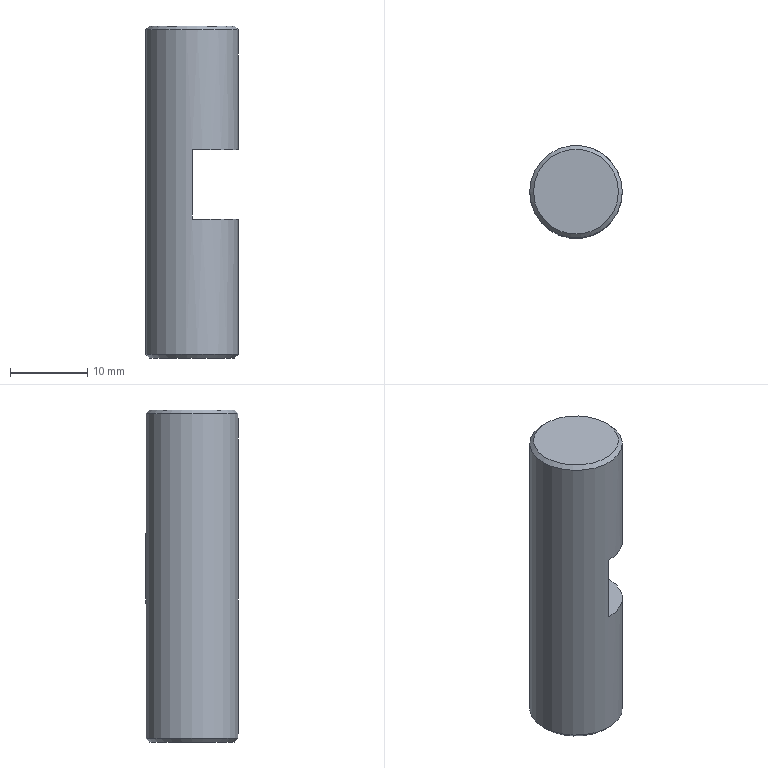Part | NX | features DATUM_CSYS 2, CHAMFER 1, CYLINDER 1, EXTRUDE 1, SKETCH 1 | 1 solid | 8 faces | box 12 x 12 x 43 mm | volume 4345 mm3 | plane 5 | cone 2 | cylinder 1 | commonest cylinder face diameters 12 x1
STEP:
#1=CARTESIAN_POINT('',(6.,0.,42.5));
#2=VERTEX_POINT('',#1);
#3=CARTESIAN_POINT('',(0.,0.,42.5));
#4=DIRECTION('',(0.,0.,1.));
#5=DIRECTION('',(1.,0.,0.));
#6=AXIS2_PLACEMENT_3D('',#3,#4,#5);
#7=CIRCLE('',#6,6.);
#8=EDGE_CURVE('',#2,#2,#7,.F.);
#9=ORIENTED_EDGE('',*,*,#8,.T.);
#10=EDGE_LOOP('',(#9));
#11=FACE_BOUND('',#10,.T.);
#12=CARTESIAN_POINT('',(-6.,0.,0.5));
#13=VERTEX_POINT('',#12);
#14=CARTESIAN_POINT('',(0.,0.,0.5));
#15=DIRECTION('',(0.,0.,-1.));
#16=DIRECTION('',(-1.,0.,0.));
#17=AXIS2_PLACEMENT_3D('',#14,#15,#16);
#18=CIRCLE('',#17,6.);
#19=EDGE_CURVE('',#13,#13,#18,.F.);
#20=ORIENTED_EDGE('',*,*,#19,.T.);
#21=EDGE_LOOP('',(#20));
#22=FACE_BOUND('',#21,.T.);
#23=CARTESIAN_POINT('',(0.,-6.,27.));
#24=VERTEX_POINT('',#23);
#25=CARTESIAN_POINT('',(0.,-6.,18.));
#26=VERTEX_POINT('',#25);
#27=CARTESIAN_POINT('',(0.,-6.,0.));
#28=DIRECTION('',(0.,0.,1.));
#29=VECTOR('',#28,1000.);
#30=LINE('',#27,#29);
#31=EDGE_CURVE('',#24,#26,#30,.F.);
#32=ORIENTED_EDGE('',*,*,#31,.F.);
#33=CARTESIAN_POINT('',(0.,6.,27.));
#34=VERTEX_POINT('',#33);
#35=CARTESIAN_POINT('',(0.,0.,27.));
#36=DIRECTION('',(0.,0.,-1.));
#37=DIRECTION('',(0.,1.,0.));
#38=AXIS2_PLACEMENT_3D('',#35,#36,#37);
#39=CIRCLE('',#38,6.);
#40=EDGE_CURVE('',#24,#34,#39,.F.);
#41=ORIENTED_EDGE('',*,*,#40,.T.);
#42=CARTESIAN_POINT('',(0.,6.,18.));
#43=VERTEX_POINT('',#42);
#44=CARTESIAN_POINT('',(0.,6.,0.));
#45=DIRECTION('',(0.,0.,1.));
#46=VECTOR('',#45,1000.);
#47=LINE('',#44,#46);
#48=EDGE_CURVE('',#43,#34,#47,.T.);
#49=ORIENTED_EDGE('',*,*,#48,.F.);
#50=CARTESIAN_POINT('',(0.,0.,18.));
#51=DIRECTION('',(0.,0.,1.));
#52=DIRECTION('',(1.,0.,0.));
#53=AXIS2_PLACEMENT_3D('',#50,#51,#52);
#54=CIRCLE('',#53,6.);
#55=EDGE_CURVE('',#43,#26,#54,.F.);
#56=ORIENTED_EDGE('',*,*,#55,.T.);
#57=EDGE_LOOP('',(#32,#41,#49,#56));
#58=FACE_BOUND('',#57,.T.);
#59=CARTESIAN_POINT('',(0.,0.,0.));
#60=DIRECTION('',(0.,0.,1.));
#61=DIRECTION('',(1.,0.,0.));
#62=AXIS2_PLACEMENT_3D('',#59,#60,#61);
#63=CYLINDRICAL_SURFACE('',#62,6.);
#64=ADVANCED_FACE('',(#11,#22,#58),#63,.T.);
#65=CARTESIAN_POINT('',(5.5,0.,43.));
#66=VERTEX_POINT('',#65);
#67=CARTESIAN_POINT('',(0.,0.,43.));
#68=DIRECTION('',(0.,0.,1.));
#69=DIRECTION('',(1.,0.,0.));
#70=AXIS2_PLACEMENT_3D('',#67,#68,#69);
#71=CIRCLE('',#70,5.5);
#72=EDGE_CURVE('',#66,#66,#71,.T.);
#73=ORIENTED_EDGE('',*,*,#72,.T.);
#74=EDGE_LOOP('',(#73));
#75=FACE_BOUND('',#74,.T.);
#76=CARTESIAN_POINT('',(0.,0.,43.));
#77=DIRECTION('',(0.,0.,1.));
#78=DIRECTION('',(1.,0.,0.));
#79=AXIS2_PLACEMENT_3D('',#76,#77,#78);
#80=PLANE('',#79);
#81=ADVANCED_FACE('',(#75),#80,.T.);
#82=CARTESIAN_POINT('',(-5.5,0.,0.));
#83=VERTEX_POINT('',#82);
#84=CARTESIAN_POINT('',(0.,0.,0.));
#85=DIRECTION('',(0.,0.,-1.));
#86=DIRECTION('',(-1.,0.,0.));
#87=AXIS2_PLACEMENT_3D('',#84,#85,#86);
#88=CIRCLE('',#87,5.5);
#89=EDGE_CURVE('',#83,#83,#88,.T.);
#90=ORIENTED_EDGE('',*,*,#89,.T.);
#91=EDGE_LOOP('',(#90));
#92=FACE_BOUND('',#91,.T.);
#93=CARTESIAN_POINT('',(0.,0.,0.));
#94=DIRECTION('',(0.,0.,-1.));
#95=DIRECTION('',(-1.,0.,0.));
#96=AXIS2_PLACEMENT_3D('',#93,#94,#95);
#97=PLANE('',#96);
#98=ADVANCED_FACE('',(#92),#97,.T.);
#99=ORIENTED_EDGE('',*,*,#72,.F.);
#100=EDGE_LOOP('',(#99));
#101=FACE_BOUND('',#100,.T.);
#102=ORIENTED_EDGE('',*,*,#8,.F.);
#103=EDGE_LOOP('',(#102));
#104=FACE_BOUND('',#103,.T.);
#105=CARTESIAN_POINT('',(0.,0.,42.5));
#106=DIRECTION('',(0.,0.,-1.));
#107=DIRECTION('',(-1.,0.,0.));
#108=AXIS2_PLACEMENT_3D('',#105,#106,#107);
#109=CONICAL_SURFACE('',#108,6.,0.7854);
#110=ADVANCED_FACE('',(#101,#104),#109,.T.);
#111=ORIENTED_EDGE('',*,*,#89,.F.);
#112=EDGE_LOOP('',(#111));
#113=FACE_BOUND('',#112,.T.);
#114=ORIENTED_EDGE('',*,*,#19,.F.);
#115=EDGE_LOOP('',(#114));
#116=FACE_BOUND('',#115,.T.);
#117=CARTESIAN_POINT('',(0.,0.,0.5));
#118=DIRECTION('',(0.,0.,1.));
#119=DIRECTION('',(1.,0.,0.));
#120=AXIS2_PLACEMENT_3D('',#117,#118,#119);
#121=CONICAL_SURFACE('',#120,6.,0.7854);
#122=ADVANCED_FACE('',(#113,#116),#121,.T.);
#123=CARTESIAN_POINT('',(0.,-17.217,27.));
#124=DIRECTION('',(0.,1.,0.));
#125=VECTOR('',#124,1000.);
#126=LINE('',#123,#125);
#127=EDGE_CURVE('',#34,#24,#126,.F.);
#128=ORIENTED_EDGE('',*,*,#127,.F.);
#129=ORIENTED_EDGE('',*,*,#40,.F.);
#130=EDGE_LOOP('',(#128,#129));
#131=FACE_BOUND('',#130,.T.);
#132=CARTESIAN_POINT('',(0.,-17.217,27.));
#133=DIRECTION('',(0.,0.,-1.));
#134=DIRECTION('',(0.,1.,0.));
#135=AXIS2_PLACEMENT_3D('',#132,#133,#134);
#136=PLANE('',#135);
#137=ADVANCED_FACE('',(#131),#136,.T.);
#138=ORIENTED_EDGE('',*,*,#55,.F.);
#139=CARTESIAN_POINT('',(0.,18.,18.));
#140=DIRECTION('',(0.,-1.,0.));
#141=VECTOR('',#140,1000.);
#142=LINE('',#139,#141);
#143=EDGE_CURVE('',#26,#43,#142,.F.);
#144=ORIENTED_EDGE('',*,*,#143,.F.);
#145=EDGE_LOOP('',(#138,#144));
#146=FACE_BOUND('',#145,.T.);
#147=CARTESIAN_POINT('',(0.,18.,18.));
#148=DIRECTION('',(0.,0.,1.));
#149=DIRECTION('',(1.,0.,0.));
#150=AXIS2_PLACEMENT_3D('',#147,#148,#149);
#151=PLANE('',#150);
#152=ADVANCED_FACE('',(#146),#151,.T.);
#153=ORIENTED_EDGE('',*,*,#31,.T.);
#154=ORIENTED_EDGE('',*,*,#143,.T.);
#155=ORIENTED_EDGE('',*,*,#48,.T.);
#156=ORIENTED_EDGE('',*,*,#127,.T.);
#157=EDGE_LOOP('',(#153,#154,#155,#156));
#158=FACE_BOUND('',#157,.T.);
#159=CARTESIAN_POINT('',(0.,0.,0.));
#160=DIRECTION('',(-1.,0.,0.));
#161=DIRECTION('',(0.,0.,1.));
#162=AXIS2_PLACEMENT_3D('',#159,#160,#161);
#163=PLANE('',#162);
#164=ADVANCED_FACE('',(#158),#163,.F.);
#165=CLOSED_SHELL('',(#64,#81,#98,#110,#122,#137,#152,#164));
#166=MANIFOLD_SOLID_BREP('',#165);
#167=(LENGTH_UNIT()NAMED_UNIT(*)SI_UNIT(.MILLI.,.METRE.));
#168=UNCERTAINTY_MEASURE_WITH_UNIT(LENGTH_MEASURE(0.00001),#167,'','');
#169=(NAMED_UNIT(*)PLANE_ANGLE_UNIT()SI_UNIT($,.RADIAN.));
#170=(NAMED_UNIT(*)SI_UNIT($,.STERADIAN.)SOLID_ANGLE_UNIT());
#171=(GEOMETRIC_REPRESENTATION_CONTEXT(3)GLOBAL_UNCERTAINTY_ASSIGNED_CONTEXT((#168))GLOBAL_UNIT_ASSIGNED_CONTEXT((#167,#169,#170))REPRESENTATION_CONTEXT('',''));
#172=ADVANCED_BREP_SHAPE_REPRESENTATION('',(#166),#171);